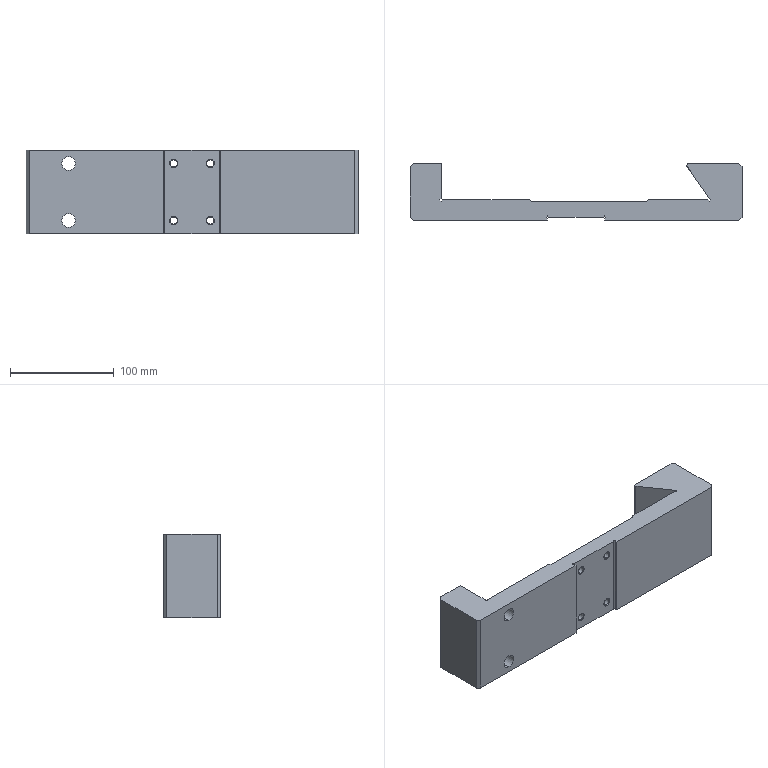Part | SolidWorks | features ICE 3, MirrorPattern 2, Chamfer 1, Extrusion 1, HoleWzd 1 | 1 solid | 55 faces | box 320 x 55 x 80 mm | volume 674156 mm3 | plane 35 | cylinder 12 | cone 8 | commonest cylinder face diameters 6.8 x8 13 x4